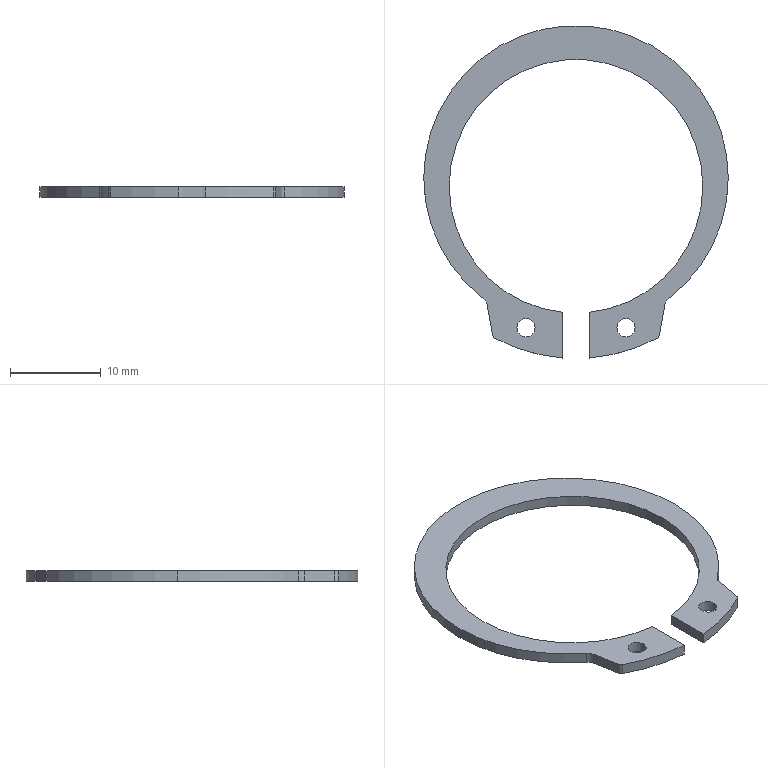Part | STEP file | circlips for shaft--type a large gb(GB_CONNECTING_PIECE_RING_RRA 30) | 1 solid | 22 faces | box 33.5 x 36.571 x 1.2 mm | volume 372.611 mm3 | cylinder 16 | plane 6 | commonest cylinder face diameters 2 x6 27.9 x3 33.5 x3 1 x2 37.9 x2